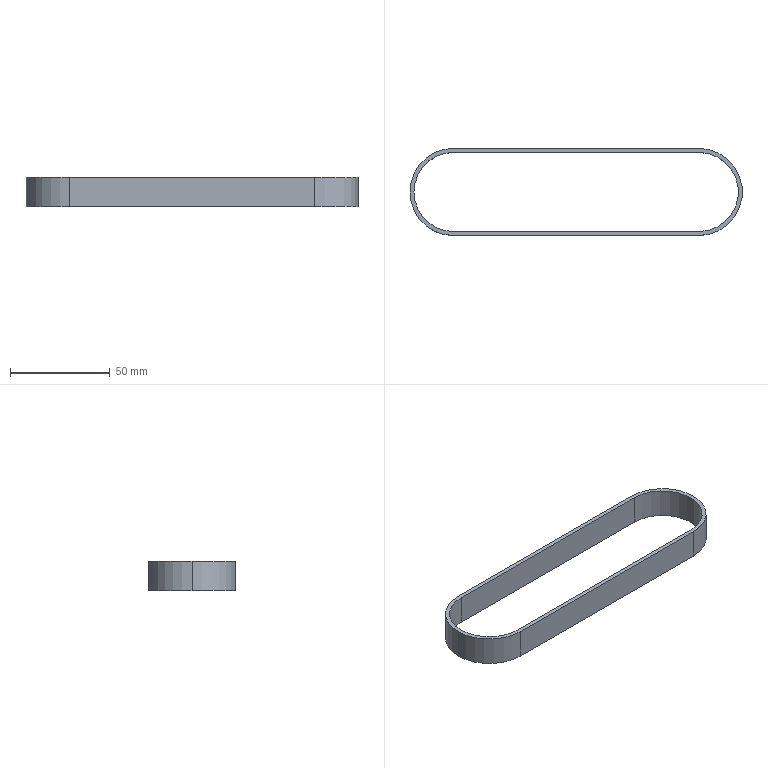Part | STEP file | C-HTBN370S5M-150 | 1 solid | 12 faces | box 166.79 x 43.79 x 15 mm | volume 11319 mm3 | cylinder 6 | plane 6 | commonest cylinder face diameters 39.79 x3 43.79 x3
STEP:
#1=CARTESIAN_POINT('',(0.,0.,0.));
#2=DIRECTION('',(0.,0.,1.));
#3=DIRECTION('',(1.,0.,0.));
#4=AXIS2_PLACEMENT_3D('',#1,#2,#3);
#5=CARTESIAN_POINT('',(-234.384,164.152,7.5));
#6=VERTEX_POINT('',#5);
#7=CARTESIAN_POINT('',(-234.384,164.152,-7.5));
#8=VERTEX_POINT('',#7);
#9=CARTESIAN_POINT('',(-234.384,164.152,7.5));
#10=DIRECTION('',(0.,0.,-1.));
#11=VECTOR('',#10,1.);
#12=LINE('',#9,#11);
#13=CARTESIAN_POINT('',(-234.384,144.257,7.5));
#14=DIRECTION('',(0.,0.,-1.));
#15=DIRECTION('',(-1.,0.,0.));
#16=AXIS2_PLACEMENT_3D('',#13,#14,#15);
#17=CYLINDRICAL_SURFACE('',#16,19.895);
#18=CARTESIAN_POINT('',(1.571,0.));
#19=DIRECTION('',(0.,1.));
#20=VECTOR('',#19,1.);
#21=LINE('',#18,#20);
#22=(GEOMETRIC_REPRESENTATION_CONTEXT(2)PARAMETRIC_REPRESENTATION_CONTEXT()REPRESENTATION_CONTEXT('',''));
#23=DEFINITIONAL_REPRESENTATION('',(#21),#22);
#24=PCURVE('',#17,#23);
#25=CARTESIAN_POINT('',(-234.384,164.152,7.5));
#26=DIRECTION('',(0.,-1.,0.));
#27=DIRECTION('',(0.,0.,-1.));
#28=AXIS2_PLACEMENT_3D('',#25,#26,#27);
#29=PLANE('',#28);
#30=CARTESIAN_POINT('',(0.,0.));
#31=DIRECTION('',(1.,0.));
#32=VECTOR('',#31,1.);
#33=LINE('',#30,#32);
#34=(GEOMETRIC_REPRESENTATION_CONTEXT(2)PARAMETRIC_REPRESENTATION_CONTEXT()REPRESENTATION_CONTEXT('',''));
#35=DEFINITIONAL_REPRESENTATION('',(#33),#34);
#36=PCURVE('',#29,#35);
#37=SURFACE_CURVE('',#12,(#24,#36),.PCURVE_S1.);
#38=EDGE_CURVE('',#6,#8,#37,.T.);
#39=ORIENTED_EDGE('',*,*,#38,.T.);
#40=CARTESIAN_POINT('',(-254.279,144.257,-7.5));
#41=VERTEX_POINT('',#40);
#42=CARTESIAN_POINT('',(-234.384,144.257,-7.5));
#43=DIRECTION('',(0.,0.,1.));
#44=DIRECTION('',(1.,0.,0.));
#45=AXIS2_PLACEMENT_3D('',#42,#43,#44);
#46=CIRCLE('',#45,19.895);
#47=CARTESIAN_POINT('',(3.142,15.));
#48=DIRECTION('',(-1.,0.));
#49=VECTOR('',#48,1.);
#50=LINE('',#47,#49);
#51=(GEOMETRIC_REPRESENTATION_CONTEXT(2)PARAMETRIC_REPRESENTATION_CONTEXT()REPRESENTATION_CONTEXT('',''));
#52=DEFINITIONAL_REPRESENTATION('',(#50),#51);
#53=PCURVE('',#17,#52);
#54=CARTESIAN_POINT('',(-234.384,144.257,-7.5));
#55=DIRECTION('',(0.,0.,1.));
#56=DIRECTION('',(1.,0.,0.));
#57=AXIS2_PLACEMENT_3D('',#54,#55,#56);
#58=PLANE('',#57);
#59=CARTESIAN_POINT('',(0.,0.));
#60=DIRECTION('',(1.,0.));
#61=AXIS2_PLACEMENT_2D('',#59,#60);
#62=CIRCLE('',#61,19.895);
#63=(GEOMETRIC_REPRESENTATION_CONTEXT(2)PARAMETRIC_REPRESENTATION_CONTEXT()REPRESENTATION_CONTEXT('',''));
#64=DEFINITIONAL_REPRESENTATION('',(#62),#63);
#65=PCURVE('',#58,#64);
#66=SURFACE_CURVE('',#46,(#53,#65),.PCURVE_S1.);
#67=EDGE_CURVE('',#8,#41,#66,.T.);
#68=ORIENTED_EDGE('',*,*,#67,.T.);
#69=CARTESIAN_POINT('',(-254.279,144.257,7.5));
#70=VERTEX_POINT('',#69);
#71=CARTESIAN_POINT('',(-254.279,144.257,7.5));
#72=DIRECTION('',(0.,0.,-1.));
#73=VECTOR('',#72,1.);
#74=LINE('',#71,#73);
#75=CARTESIAN_POINT('',(0.,0.));
#76=DIRECTION('',(0.,1.));
#77=VECTOR('',#76,1.);
#78=LINE('',#75,#77);
#79=(GEOMETRIC_REPRESENTATION_CONTEXT(2)PARAMETRIC_REPRESENTATION_CONTEXT()REPRESENTATION_CONTEXT('',''));
#80=DEFINITIONAL_REPRESENTATION('',(#78),#79);
#81=PCURVE('',#17,#80);
#82=CARTESIAN_POINT('',(-234.384,144.257,7.5));
#83=DIRECTION('',(0.,0.,-1.));
#84=DIRECTION('',(-1.,0.,0.));
#85=AXIS2_PLACEMENT_3D('',#82,#83,#84);
#86=CYLINDRICAL_SURFACE('',#85,19.895);
#87=CARTESIAN_POINT('',(6.283,0.));
#88=DIRECTION('',(0.,1.));
#89=VECTOR('',#88,1.);
#90=LINE('',#87,#89);
#91=(GEOMETRIC_REPRESENTATION_CONTEXT(2)PARAMETRIC_REPRESENTATION_CONTEXT()REPRESENTATION_CONTEXT('',''));
#92=DEFINITIONAL_REPRESENTATION('',(#90),#91);
#93=PCURVE('',#86,#92);
#94=SURFACE_CURVE('',#74,(#81,#93),.PCURVE_S1.);
#95=EDGE_CURVE('',#70,#41,#94,.T.);
#96=ORIENTED_EDGE('',*,*,#95,.F.);
#97=CARTESIAN_POINT('',(-234.384,144.257,7.5));
#98=DIRECTION('',(0.,0.,1.));
#99=DIRECTION('',(1.,0.,0.));
#100=AXIS2_PLACEMENT_3D('',#97,#98,#99);
#101=CIRCLE('',#100,19.895);
#102=CARTESIAN_POINT('',(3.142,0.));
#103=DIRECTION('',(-1.,0.));
#104=VECTOR('',#103,1.);
#105=LINE('',#102,#104);
#106=(GEOMETRIC_REPRESENTATION_CONTEXT(2)PARAMETRIC_REPRESENTATION_CONTEXT()REPRESENTATION_CONTEXT('',''));
#107=DEFINITIONAL_REPRESENTATION('',(#105),#106);
#108=PCURVE('',#17,#107);
#109=CARTESIAN_POINT('',(-234.384,144.257,7.5));
#110=DIRECTION('',(0.,0.,1.));
#111=DIRECTION('',(1.,0.,0.));
#112=AXIS2_PLACEMENT_3D('',#109,#110,#111);
#113=PLANE('',#112);
#114=CARTESIAN_POINT('',(0.,0.));
#115=DIRECTION('',(1.,0.));
#116=AXIS2_PLACEMENT_2D('',#114,#115);
#117=CIRCLE('',#116,19.895);
#118=(GEOMETRIC_REPRESENTATION_CONTEXT(2)PARAMETRIC_REPRESENTATION_CONTEXT()REPRESENTATION_CONTEXT('',''));
#119=DEFINITIONAL_REPRESENTATION('',(#117),#118);
#120=PCURVE('',#113,#119);
#121=SURFACE_CURVE('',#101,(#108,#120),.PCURVE_S1.);
#122=EDGE_CURVE('',#6,#70,#121,.T.);
#123=ORIENTED_EDGE('',*,*,#122,.F.);
#124=EDGE_LOOP('',(#39,#68,#96,#123));
#125=FACE_BOUND('',#124,.F.);
#126=ADVANCED_FACE('',(#125),#17,.F.);
#127=CARTESIAN_POINT('',(-256.279,144.257,7.5));
#128=VERTEX_POINT('',#127);
#129=CARTESIAN_POINT('',(-234.384,122.362,7.5));
#130=VERTEX_POINT('',#129);
#131=CARTESIAN_POINT('',(-234.384,144.257,7.5));
#132=DIRECTION('',(0.,0.,1.));
#133=DIRECTION('',(1.,0.,0.));
#134=AXIS2_PLACEMENT_3D('',#131,#132,#133);
#135=CIRCLE('',#134,21.895);
#136=CARTESIAN_POINT('',(-234.384,144.257,7.5));
#137=DIRECTION('',(0.,0.,-1.));
#138=DIRECTION('',(-1.,0.,0.));
#139=AXIS2_PLACEMENT_3D('',#136,#137,#138);
#140=CYLINDRICAL_SURFACE('',#139,21.895);
#141=CARTESIAN_POINT('',(9.425,0.));
#142=DIRECTION('',(-1.,0.));
#143=VECTOR('',#142,1.);
#144=LINE('',#141,#143);
#145=(GEOMETRIC_REPRESENTATION_CONTEXT(2)PARAMETRIC_REPRESENTATION_CONTEXT()REPRESENTATION_CONTEXT('',''));
#146=DEFINITIONAL_REPRESENTATION('',(#144),#145);
#147=PCURVE('',#140,#146);
#148=CARTESIAN_POINT('',(0.,0.));
#149=DIRECTION('',(1.,0.));
#150=AXIS2_PLACEMENT_2D('',#148,#149);
#151=CIRCLE('',#150,21.895);
#152=(GEOMETRIC_REPRESENTATION_CONTEXT(2)PARAMETRIC_REPRESENTATION_CONTEXT()REPRESENTATION_CONTEXT('',''));
#153=DEFINITIONAL_REPRESENTATION('',(#151),#152);
#154=PCURVE('',#113,#153);
#155=SURFACE_CURVE('',#135,(#147,#154),.PCURVE_S1.);
#156=EDGE_CURVE('',#128,#130,#155,.T.);
#157=ORIENTED_EDGE('',*,*,#156,.F.);
#158=CARTESIAN_POINT('',(-256.279,144.257,-7.5));
#159=VERTEX_POINT('',#158);
#160=CARTESIAN_POINT('',(-256.279,144.257,7.5));
#161=DIRECTION('',(0.,0.,-1.));
#162=VECTOR('',#161,1.);
#163=LINE('',#160,#162);
#164=CARTESIAN_POINT('',(6.283,0.));
#165=DIRECTION('',(0.,1.));
#166=VECTOR('',#165,1.);
#167=LINE('',#164,#166);
#168=(GEOMETRIC_REPRESENTATION_CONTEXT(2)PARAMETRIC_REPRESENTATION_CONTEXT()REPRESENTATION_CONTEXT('',''));
#169=DEFINITIONAL_REPRESENTATION('',(#167),#168);
#170=PCURVE('',#140,#169);
#171=CARTESIAN_POINT('',(-234.384,144.257,7.5));
#172=DIRECTION('',(0.,0.,-1.));
#173=DIRECTION('',(-1.,0.,0.));
#174=AXIS2_PLACEMENT_3D('',#171,#172,#173);
#175=CYLINDRICAL_SURFACE('',#174,21.895);
#176=CARTESIAN_POINT('',(0.,0.));
#177=DIRECTION('',(0.,1.));
#178=VECTOR('',#177,1.);
#179=LINE('',#176,#178);
#180=(GEOMETRIC_REPRESENTATION_CONTEXT(2)PARAMETRIC_REPRESENTATION_CONTEXT()REPRESENTATION_CONTEXT('',''));
#181=DEFINITIONAL_REPRESENTATION('',(#179),#180);
#182=PCURVE('',#175,#181);
#183=SURFACE_CURVE('',#163,(#170,#182),.PCURVE_S1.);
#184=EDGE_CURVE('',#128,#159,#183,.T.);
#185=ORIENTED_EDGE('',*,*,#184,.T.);
#186=CARTESIAN_POINT('',(-234.384,122.362,-7.5));
#187=VERTEX_POINT('',#186);
#188=CARTESIAN_POINT('',(-234.384,144.257,-7.5));
#189=DIRECTION('',(0.,0.,1.));
#190=DIRECTION('',(1.,0.,0.));
#191=AXIS2_PLACEMENT_3D('',#188,#189,#190);
#192=CIRCLE('',#191,21.895);
#193=CARTESIAN_POINT('',(9.425,15.));
#194=DIRECTION('',(-1.,0.));
#195=VECTOR('',#194,1.);
#196=LINE('',#193,#195);
#197=(GEOMETRIC_REPRESENTATION_CONTEXT(2)PARAMETRIC_REPRESENTATION_CONTEXT()REPRESENTATION_CONTEXT('',''));
#198=DEFINITIONAL_REPRESENTATION('',(#196),#197);
#199=PCURVE('',#140,#198);
#200=CARTESIAN_POINT('',(0.,0.));
#201=DIRECTION('',(1.,0.));
#202=AXIS2_PLACEMENT_2D('',#200,#201);
#203=CIRCLE('',#202,21.895);
#204=(GEOMETRIC_REPRESENTATION_CONTEXT(2)PARAMETRIC_REPRESENTATION_CONTEXT()REPRESENTATION_CONTEXT('',''));
#205=DEFINITIONAL_REPRESENTATION('',(#203),#204);
#206=PCURVE('',#58,#205);
#207=SURFACE_CURVE('',#192,(#199,#206),.PCURVE_S1.);
#208=EDGE_CURVE('',#159,#187,#207,.T.);
#209=ORIENTED_EDGE('',*,*,#208,.T.);
#210=CARTESIAN_POINT('',(-234.384,122.362,7.5));
#211=DIRECTION('',(0.,0.,-1.));
#212=VECTOR('',#211,1.);
#213=LINE('',#210,#212);
#214=CARTESIAN_POINT('',(4.712,0.));
#215=DIRECTION('',(0.,1.));
#216=VECTOR('',#215,1.);
#217=LINE('',#214,#216);
#218=(GEOMETRIC_REPRESENTATION_CONTEXT(2)PARAMETRIC_REPRESENTATION_CONTEXT()REPRESENTATION_CONTEXT('',''));
#219=DEFINITIONAL_REPRESENTATION('',(#217),#218);
#220=PCURVE('',#140,#219);
#221=CARTESIAN_POINT('',(-234.384,122.362,7.5));
#222=DIRECTION('',(0.,1.,0.));
#223=DIRECTION('',(-1.,0.,0.));
#224=AXIS2_PLACEMENT_3D('',#221,#222,#223);
#225=PLANE('',#224);
#226=CARTESIAN_POINT('',(0.,0.));
#227=DIRECTION('',(0.,-1.));
#228=VECTOR('',#227,1.);
#229=LINE('',#226,#228);
#230=(GEOMETRIC_REPRESENTATION_CONTEXT(2)PARAMETRIC_REPRESENTATION_CONTEXT()REPRESENTATION_CONTEXT('',''));
#231=DEFINITIONAL_REPRESENTATION('',(#229),#230);
#232=PCURVE('',#225,#231);
#233=SURFACE_CURVE('',#213,(#220,#232),.PCURVE_S1.);
#234=EDGE_CURVE('',#130,#187,#233,.T.);
#235=ORIENTED_EDGE('',*,*,#234,.F.);
#236=EDGE_LOOP('',(#157,#185,#209,#235));
#237=FACE_BOUND('',#236,.T.);
#238=ADVANCED_FACE('',(#237),#140,.T.);
#239=CARTESIAN_POINT('',(-234.384,166.152,7.5));
#240=VERTEX_POINT('',#239);
#241=CARTESIAN_POINT('',(-234.384,144.257,7.5));
#242=DIRECTION('',(0.,0.,1.));
#243=DIRECTION('',(1.,0.,0.));
#244=AXIS2_PLACEMENT_3D('',#241,#242,#243);
#245=CIRCLE('',#244,21.895);
#246=CARTESIAN_POINT('',(0.,0.));
#247=DIRECTION('',(1.,0.));
#248=AXIS2_PLACEMENT_2D('',#246,#247);
#249=CIRCLE('',#248,21.895);
#250=(GEOMETRIC_REPRESENTATION_CONTEXT(2)PARAMETRIC_REPRESENTATION_CONTEXT()REPRESENTATION_CONTEXT('',''));
#251=DEFINITIONAL_REPRESENTATION('',(#249),#250);
#252=PCURVE('',#113,#251);
#253=CARTESIAN_POINT('',(3.142,0.));
#254=DIRECTION('',(-1.,0.));
#255=VECTOR('',#254,1.);
#256=LINE('',#253,#255);
#257=(GEOMETRIC_REPRESENTATION_CONTEXT(2)PARAMETRIC_REPRESENTATION_CONTEXT()REPRESENTATION_CONTEXT('',''));
#258=DEFINITIONAL_REPRESENTATION('',(#256),#257);
#259=PCURVE('',#175,#258);
#260=SURFACE_CURVE('',#245,(#252,#259),.PCURVE_S1.);
#261=EDGE_CURVE('',#240,#128,#260,.T.);
#262=ORIENTED_EDGE('',*,*,#261,.T.);
#263=ORIENTED_EDGE('',*,*,#156,.T.);
#264=CARTESIAN_POINT('',(-111.384,122.362,7.5));
#265=VERTEX_POINT('',#264);
#266=CARTESIAN_POINT('',(-234.384,122.362,7.5));
#267=DIRECTION('',(1.,0.,0.));
#268=VECTOR('',#267,1.);
#269=LINE('',#266,#268);
#270=CARTESIAN_POINT('',(0.,-21.895));
#271=DIRECTION('',(1.,0.));
#272=VECTOR('',#271,1.);
#273=LINE('',#270,#272);
#274=(GEOMETRIC_REPRESENTATION_CONTEXT(2)PARAMETRIC_REPRESENTATION_CONTEXT()REPRESENTATION_CONTEXT('',''));
#275=DEFINITIONAL_REPRESENTATION('',(#273),#274);
#276=PCURVE('',#113,#275);
#277=CARTESIAN_POINT('',(0.,0.));
#278=DIRECTION('',(-1.,0.));
#279=VECTOR('',#278,1.);
#280=LINE('',#277,#279);
#281=(GEOMETRIC_REPRESENTATION_CONTEXT(2)PARAMETRIC_REPRESENTATION_CONTEXT()REPRESENTATION_CONTEXT('',''));
#282=DEFINITIONAL_REPRESENTATION('',(#280),#281);
#283=PCURVE('',#225,#282);
#284=SURFACE_CURVE('',#269,(#276,#283),.PCURVE_S1.);
#285=EDGE_CURVE('',#130,#265,#284,.T.);
#286=ORIENTED_EDGE('',*,*,#285,.T.);
#287=CARTESIAN_POINT('',(-111.384,166.152,7.5));
#288=VERTEX_POINT('',#287);
#289=CARTESIAN_POINT('',(-111.384,144.257,7.5));
#290=DIRECTION('',(0.,0.,1.));
#291=DIRECTION('',(1.,0.,0.));
#292=AXIS2_PLACEMENT_3D('',#289,#290,#291);
#293=CIRCLE('',#292,21.895);
#294=CARTESIAN_POINT('',(123.,0.));
#295=DIRECTION('',(1.,0.));
#296=AXIS2_PLACEMENT_2D('',#294,#295);
#297=CIRCLE('',#296,21.895);
#298=(GEOMETRIC_REPRESENTATION_CONTEXT(2)PARAMETRIC_REPRESENTATION_CONTEXT()REPRESENTATION_CONTEXT('',''));
#299=DEFINITIONAL_REPRESENTATION('',(#297),#298);
#300=PCURVE('',#113,#299);
#301=CARTESIAN_POINT('',(-111.384,144.257,7.5));
#302=DIRECTION('',(0.,0.,-1.));
#303=DIRECTION('',(-1.,0.,0.));
#304=AXIS2_PLACEMENT_3D('',#301,#302,#303);
#305=CYLINDRICAL_SURFACE('',#304,21.895);
#306=CARTESIAN_POINT('',(9.425,0.));
#307=DIRECTION('',(-1.,0.));
#308=VECTOR('',#307,1.);
#309=LINE('',#306,#308);
#310=(GEOMETRIC_REPRESENTATION_CONTEXT(2)PARAMETRIC_REPRESENTATION_CONTEXT()REPRESENTATION_CONTEXT('',''));
#311=DEFINITIONAL_REPRESENTATION('',(#309),#310);
#312=PCURVE('',#305,#311);
#313=SURFACE_CURVE('',#293,(#300,#312),.PCURVE_S1.);
#314=EDGE_CURVE('',#265,#288,#313,.T.);
#315=ORIENTED_EDGE('',*,*,#314,.T.);
#316=CARTESIAN_POINT('',(-234.384,166.152,7.5));
#317=DIRECTION('',(-1.,0.,0.));
#318=VECTOR('',#317,1.);
#319=LINE('',#316,#318);
#320=CARTESIAN_POINT('',(0.,21.895));
#321=DIRECTION('',(-1.,0.));
#322=VECTOR('',#321,1.);
#323=LINE('',#320,#322);
#324=(GEOMETRIC_REPRESENTATION_CONTEXT(2)PARAMETRIC_REPRESENTATION_CONTEXT()REPRESENTATION_CONTEXT('',''));
#325=DEFINITIONAL_REPRESENTATION('',(#323),#324);
#326=PCURVE('',#113,#325);
#327=CARTESIAN_POINT('',(-234.384,166.152,7.5));
#328=DIRECTION('',(0.,-1.,0.));
#329=DIRECTION('',(0.,0.,-1.));
#330=AXIS2_PLACEMENT_3D('',#327,#328,#329);
#331=PLANE('',#330);
#332=CARTESIAN_POINT('',(0.,0.));
#333=DIRECTION('',(0.,-1.));
#334=VECTOR('',#333,1.);
#335=LINE('',#332,#334);
#336=(GEOMETRIC_REPRESENTATION_CONTEXT(2)PARAMETRIC_REPRESENTATION_CONTEXT()REPRESENTATION_CONTEXT('',''));
#337=DEFINITIONAL_REPRESENTATION('',(#335),#336);
#338=PCURVE('',#331,#337);
#339=SURFACE_CURVE('',#319,(#326,#338),.PCURVE_S1.);
#340=EDGE_CURVE('',#288,#240,#339,.T.);
#341=ORIENTED_EDGE('',*,*,#340,.T.);
#342=EDGE_LOOP('',(#262,#263,#286,#315,#341));
#343=FACE_BOUND('',#342,.T.);
#344=CARTESIAN_POINT('',(-234.384,124.362,7.5));
#345=VERTEX_POINT('',#344);
#346=CARTESIAN_POINT('',(-111.384,124.362,7.5));
#347=VERTEX_POINT('',#346);
#348=CARTESIAN_POINT('',(-234.384,124.362,7.5));
#349=DIRECTION('',(1.,0.,0.));
#350=VECTOR('',#349,1.);
#351=LINE('',#348,#350);
#352=CARTESIAN_POINT('',(0.,-19.895));
#353=DIRECTION('',(1.,0.));
#354=VECTOR('',#353,1.);
#355=LINE('',#352,#354);
#356=(GEOMETRIC_REPRESENTATION_CONTEXT(2)PARAMETRIC_REPRESENTATION_CONTEXT()REPRESENTATION_CONTEXT('',''));
#357=DEFINITIONAL_REPRESENTATION('',(#355),#356);
#358=PCURVE('',#113,#357);
#359=CARTESIAN_POINT('',(-234.384,124.362,7.5));
#360=DIRECTION('',(0.,1.,0.));
#361=DIRECTION('',(-1.,0.,0.));
#362=AXIS2_PLACEMENT_3D('',#359,#360,#361);
#363=PLANE('',#362);
#364=CARTESIAN_POINT('',(0.,0.));
#365=DIRECTION('',(-1.,0.));
#366=VECTOR('',#365,1.);
#367=LINE('',#364,#366);
#368=(GEOMETRIC_REPRESENTATION_CONTEXT(2)PARAMETRIC_REPRESENTATION_CONTEXT()REPRESENTATION_CONTEXT('',''));
#369=DEFINITIONAL_REPRESENTATION('',(#367),#368);
#370=PCURVE('',#363,#369);
#371=SURFACE_CURVE('',#351,(#358,#370),.PCURVE_S1.);
#372=EDGE_CURVE('',#345,#347,#371,.T.);
#373=ORIENTED_EDGE('',*,*,#372,.F.);
#374=CARTESIAN_POINT('',(-234.384,144.257,7.5));
#375=DIRECTION('',(0.,0.,1.));
#376=DIRECTION('',(1.,0.,0.));
#377=AXIS2_PLACEMENT_3D('',#374,#375,#376);
#378=CIRCLE('',#377,19.895);
#379=CARTESIAN_POINT('',(0.,0.));
#380=DIRECTION('',(1.,0.));
#381=AXIS2_PLACEMENT_2D('',#379,#380);
#382=CIRCLE('',#381,19.895);
#383=(GEOMETRIC_REPRESENTATION_CONTEXT(2)PARAMETRIC_REPRESENTATION_CONTEXT()REPRESENTATION_CONTEXT('',''));
#384=DEFINITIONAL_REPRESENTATION('',(#382),#383);
#385=PCURVE('',#113,#384);
#386=CARTESIAN_POINT('',(9.425,0.));
#387=DIRECTION('',(-1.,0.));
#388=VECTOR('',#387,1.);
#389=LINE('',#386,#388);
#390=(GEOMETRIC_REPRESENTATION_CONTEXT(2)PARAMETRIC_REPRESENTATION_CONTEXT()REPRESENTATION_CONTEXT('',''));
#391=DEFINITIONAL_REPRESENTATION('',(#389),#390);
#392=PCURVE('',#86,#391);
#393=SURFACE_CURVE('',#378,(#385,#392),.PCURVE_S1.);
#394=EDGE_CURVE('',#70,#345,#393,.T.);
#395=ORIENTED_EDGE('',*,*,#394,.F.);
#396=ORIENTED_EDGE('',*,*,#122,.F.);
#397=CARTESIAN_POINT('',(-111.384,164.152,7.5));
#398=VERTEX_POINT('',#397);
#399=CARTESIAN_POINT('',(-234.384,164.152,7.5));
#400=DIRECTION('',(-1.,0.,0.));
#401=VECTOR('',#400,1.);
#402=LINE('',#399,#401);
#403=CARTESIAN_POINT('',(0.,19.895));
#404=DIRECTION('',(-1.,0.));
#405=VECTOR('',#404,1.);
#406=LINE('',#403,#405);
#407=(GEOMETRIC_REPRESENTATION_CONTEXT(2)PARAMETRIC_REPRESENTATION_CONTEXT()REPRESENTATION_CONTEXT('',''));
#408=DEFINITIONAL_REPRESENTATION('',(#406),#407);
#409=PCURVE('',#113,#408);
#410=CARTESIAN_POINT('',(0.,0.));
#411=DIRECTION('',(0.,-1.));
#412=VECTOR('',#411,1.);
#413=LINE('',#410,#412);
#414=(GEOMETRIC_REPRESENTATION_CONTEXT(2)PARAMETRIC_REPRESENTATION_CONTEXT()REPRESENTATION_CONTEXT('',''));
#415=DEFINITIONAL_REPRESENTATION('',(#413),#414);
#416=PCURVE('',#29,#415);
#417=SURFACE_CURVE('',#402,(#409,#416),.PCURVE_S1.);
#418=EDGE_CURVE('',#398,#6,#417,.T.);
#419=ORIENTED_EDGE('',*,*,#418,.F.);
#420=CARTESIAN_POINT('',(-111.384,144.257,7.5));
#421=DIRECTION('',(0.,0.,1.));
#422=DIRECTION('',(1.,0.,0.));
#423=AXIS2_PLACEMENT_3D('',#420,#421,#422);
#424=CIRCLE('',#423,19.895);
#425=CARTESIAN_POINT('',(123.,0.));
#426=DIRECTION('',(1.,0.));
#427=AXIS2_PLACEMENT_2D('',#425,#426);
#428=CIRCLE('',#427,19.895);
#429=(GEOMETRIC_REPRESENTATION_CONTEXT(2)PARAMETRIC_REPRESENTATION_CONTEXT()REPRESENTATION_CONTEXT('',''));
#430=DEFINITIONAL_REPRESENTATION('',(#428),#429);
#431=PCURVE('',#113,#430);
#432=CARTESIAN_POINT('',(-111.384,144.257,7.5));
#433=DIRECTION('',(0.,0.,-1.));
#434=DIRECTION('',(-1.,0.,0.));
#435=AXIS2_PLACEMENT_3D('',#432,#433,#434);
#436=CYLINDRICAL_SURFACE('',#435,19.895);
#437=CARTESIAN_POINT('',(9.425,0.));
#438=DIRECTION('',(-1.,0.));
#439=VECTOR('',#438,1.);
#440=LINE('',#437,#439);
#441=(GEOMETRIC_REPRESENTATION_CONTEXT(2)PARAMETRIC_REPRESENTATION_CONTEXT()REPRESENTATION_CONTEXT('',''));
#442=DEFINITIONAL_REPRESENTATION('',(#440),#441);
#443=PCURVE('',#436,#442);
#444=SURFACE_CURVE('',#424,(#431,#443),.PCURVE_S1.);
#445=EDGE_CURVE('',#347,#398,#444,.T.);
#446=ORIENTED_EDGE('',*,*,#445,.F.);
#447=EDGE_LOOP('',(#373,#395,#396,#419,#446));
#448=FACE_BOUND('',#447,.T.);
#449=ADVANCED_FACE('',(#343,#448),#113,.T.);
#450=CARTESIAN_POINT('',(-234.384,166.152,-7.5));
#451=VERTEX_POINT('',#450);
#452=CARTESIAN_POINT('',(-234.384,144.257,-7.5));
#453=DIRECTION('',(0.,0.,1.));
#454=DIRECTION('',(1.,0.,0.));
#455=AXIS2_PLACEMENT_3D('',#452,#453,#454);
#456=CIRCLE('',#455,21.895);
#457=CARTESIAN_POINT('',(0.,0.));
#458=DIRECTION('',(1.,0.));
#459=AXIS2_PLACEMENT_2D('',#457,#458);
#460=CIRCLE('',#459,21.895);
#461=(GEOMETRIC_REPRESENTATION_CONTEXT(2)PARAMETRIC_REPRESENTATION_CONTEXT()REPRESENTATION_CONTEXT('',''));
#462=DEFINITIONAL_REPRESENTATION('',(#460),#461);
#463=PCURVE('',#58,#462);
#464=CARTESIAN_POINT('',(3.142,15.));
#465=DIRECTION('',(-1.,0.));
#466=VECTOR('',#465,1.);
#467=LINE('',#464,#466);
#468=(GEOMETRIC_REPRESENTATION_CONTEXT(2)PARAMETRIC_REPRESENTATION_CONTEXT()REPRESENTATION_CONTEXT('',''));
#469=DEFINITIONAL_REPRESENTATION('',(#467),#468);
#470=PCURVE('',#175,#469);
#471=SURFACE_CURVE('',#456,(#463,#470),.PCURVE_S1.);
#472=EDGE_CURVE('',#451,#159,#471,.T.);
#473=ORIENTED_EDGE('',*,*,#472,.F.);
#474=CARTESIAN_POINT('',(-111.384,166.152,-7.5));
#475=VERTEX_POINT('',#474);
#476=CARTESIAN_POINT('',(-234.384,166.152,-7.5));
#477=DIRECTION('',(-1.,0.,0.));
#478=VECTOR('',#477,1.);
#479=LINE('',#476,#478);
#480=CARTESIAN_POINT('',(0.,21.895));
#481=DIRECTION('',(-1.,0.));
#482=VECTOR('',#481,1.);
#483=LINE('',#480,#482);
#484=(GEOMETRIC_REPRESENTATION_CONTEXT(2)PARAMETRIC_REPRESENTATION_CONTEXT()REPRESENTATION_CONTEXT('',''));
#485=DEFINITIONAL_REPRESENTATION('',(#483),#484);
#486=PCURVE('',#58,#485);
#487=CARTESIAN_POINT('',(15.,0.));
#488=DIRECTION('',(0.,-1.));
#489=VECTOR('',#488,1.);
#490=LINE('',#487,#489);
#491=(GEOMETRIC_REPRESENTATION_CONTEXT(2)PARAMETRIC_REPRESENTATION_CONTEXT()REPRESENTATION_CONTEXT('',''));
#492=DEFINITIONAL_REPRESENTATION('',(#490),#491);
#493=PCURVE('',#331,#492);
#494=SURFACE_CURVE('',#479,(#486,#493),.PCURVE_S1.);
#495=EDGE_CURVE('',#475,#451,#494,.T.);
#496=ORIENTED_EDGE('',*,*,#495,.F.);
#497=CARTESIAN_POINT('',(-111.384,122.362,-7.5));
#498=VERTEX_POINT('',#497);
#499=CARTESIAN_POINT('',(-111.384,144.257,-7.5));
#500=DIRECTION('',(0.,0.,1.));
#501=DIRECTION('',(1.,0.,0.));
#502=AXIS2_PLACEMENT_3D('',#499,#500,#501);
#503=CIRCLE('',#502,21.895);
#504=CARTESIAN_POINT('',(123.,0.));
#505=DIRECTION('',(1.,0.));
#506=AXIS2_PLACEMENT_2D('',#504,#505);
#507=CIRCLE('',#506,21.895);
#508=(GEOMETRIC_REPRESENTATION_CONTEXT(2)PARAMETRIC_REPRESENTATION_CONTEXT()REPRESENTATION_CONTEXT('',''));
#509=DEFINITIONAL_REPRESENTATION('',(#507),#508);
#510=PCURVE('',#58,#509);
#511=CARTESIAN_POINT('',(9.425,15.));
#512=DIRECTION('',(-1.,0.));
#513=VECTOR('',#512,1.);
#514=LINE('',#511,#513);
#515=(GEOMETRIC_REPRESENTATION_CONTEXT(2)PARAMETRIC_REPRESENTATION_CONTEXT()REPRESENTATION_CONTEXT('',''));
#516=DEFINITIONAL_REPRESENTATION('',(#514),#515);
#517=PCURVE('',#305,#516);
#518=SURFACE_CURVE('',#503,(#510,#517),.PCURVE_S1.);
#519=EDGE_CURVE('',#498,#475,#518,.T.);
#520=ORIENTED_EDGE('',*,*,#519,.F.);
#521=CARTESIAN_POINT('',(-234.384,122.362,-7.5));
#522=DIRECTION('',(1.,0.,0.));
#523=VECTOR('',#522,1.);
#524=LINE('',#521,#523);
#525=CARTESIAN_POINT('',(0.,-21.895));
#526=DIRECTION('',(1.,0.));
#527=VECTOR('',#526,1.);
#528=LINE('',#525,#527);
#529=(GEOMETRIC_REPRESENTATION_CONTEXT(2)PARAMETRIC_REPRESENTATION_CONTEXT()REPRESENTATION_CONTEXT('',''));
#530=DEFINITIONAL_REPRESENTATION('',(#528),#529);
#531=PCURVE('',#58,#530);
#532=CARTESIAN_POINT('',(0.,-15.));
#533=DIRECTION('',(-1.,0.));
#534=VECTOR('',#533,1.);
#535=LINE('',#532,#534);
#536=(GEOMETRIC_REPRESENTATION_CONTEXT(2)PARAMETRIC_REPRESENTATION_CONTEXT()REPRESENTATION_CONTEXT('',''));
#537=DEFINITIONAL_REPRESENTATION('',(#535),#536);
#538=PCURVE('',#225,#537);
#539=SURFACE_CURVE('',#524,(#531,#538),.PCURVE_S1.);
#540=EDGE_CURVE('',#187,#498,#539,.T.);
#541=ORIENTED_EDGE('',*,*,#540,.F.);
#542=ORIENTED_EDGE('',*,*,#208,.F.);
#543=EDGE_LOOP('',(#473,#496,#520,#541,#542));
#544=FACE_BOUND('',#543,.T.);
#545=ORIENTED_EDGE('',*,*,#67,.T.);
#546=CARTESIAN_POINT('',(-234.384,124.362,-7.5));
#547=VERTEX_POINT('',#546);
#548=CARTESIAN_POINT('',(-234.384,144.257,-7.5));
#549=DIRECTION('',(0.,0.,1.));
#550=DIRECTION('',(1.,0.,0.));
#551=AXIS2_PLACEMENT_3D('',#548,#549,#550);
#552=CIRCLE('',#551,19.895);
#553=CARTESIAN_POINT('',(0.,0.));
#554=DIRECTION('',(1.,0.));
#555=AXIS2_PLACEMENT_2D('',#553,#554);
#556=CIRCLE('',#555,19.895);
#557=(GEOMETRIC_REPRESENTATION_CONTEXT(2)PARAMETRIC_REPRESENTATION_CONTEXT()REPRESENTATION_CONTEXT('',''));
#558=DEFINITIONAL_REPRESENTATION('',(#556),#557);
#559=PCURVE('',#58,#558);
#560=CARTESIAN_POINT('',(9.425,15.));
#561=DIRECTION('',(-1.,0.));
#562=VECTOR('',#561,1.);
#563=LINE('',#560,#562);
#564=(GEOMETRIC_REPRESENTATION_CONTEXT(2)PARAMETRIC_REPRESENTATION_CONTEXT()REPRESENTATION_CONTEXT('',''));
#565=DEFINITIONAL_REPRESENTATION('',(#563),#564);
#566=PCURVE('',#86,#565);
#567=SURFACE_CURVE('',#552,(#559,#566),.PCURVE_S1.);
#568=EDGE_CURVE('',#41,#547,#567,.T.);
#569=ORIENTED_EDGE('',*,*,#568,.T.);
#570=CARTESIAN_POINT('',(-111.384,124.362,-7.5));
#571=VERTEX_POINT('',#570);
#572=CARTESIAN_POINT('',(-234.384,124.362,-7.5));
#573=DIRECTION('',(1.,0.,0.));
#574=VECTOR('',#573,1.);
#575=LINE('',#572,#574);
#576=CARTESIAN_POINT('',(0.,-19.895));
#577=DIRECTION('',(1.,0.));
#578=VECTOR('',#577,1.);
#579=LINE('',#576,#578);
#580=(GEOMETRIC_REPRESENTATION_CONTEXT(2)PARAMETRIC_REPRESENTATION_CONTEXT()REPRESENTATION_CONTEXT('',''));
#581=DEFINITIONAL_REPRESENTATION('',(#579),#580);
#582=PCURVE('',#58,#581);
#583=CARTESIAN_POINT('',(0.,-15.));
#584=DIRECTION('',(-1.,0.));
#585=VECTOR('',#584,1.);
#586=LINE('',#583,#585);
#587=(GEOMETRIC_REPRESENTATION_CONTEXT(2)PARAMETRIC_REPRESENTATION_CONTEXT()REPRESENTATION_CONTEXT('',''));
#588=DEFINITIONAL_REPRESENTATION('',(#586),#587);
#589=PCURVE('',#363,#588);
#590=SURFACE_CURVE('',#575,(#582,#589),.PCURVE_S1.);
#591=EDGE_CURVE('',#547,#571,#590,.T.);
#592=ORIENTED_EDGE('',*,*,#591,.T.);
#593=CARTESIAN_POINT('',(-111.384,164.152,-7.5));
#594=VERTEX_POINT('',#593);
#595=CARTESIAN_POINT('',(-111.384,144.257,-7.5));
#596=DIRECTION('',(0.,0.,1.));
#597=DIRECTION('',(1.,0.,0.));
#598=AXIS2_PLACEMENT_3D('',#595,#596,#597);
#599=CIRCLE('',#598,19.895);
#600=CARTESIAN_POINT('',(123.,0.));
#601=DIRECTION('',(1.,0.));
#602=AXIS2_PLACEMENT_2D('',#600,#601);
#603=CIRCLE('',#602,19.895);
#604=(GEOMETRIC_REPRESENTATION_CONTEXT(2)PARAMETRIC_REPRESENTATION_CONTEXT()REPRESENTATION_CONTEXT('',''));
#605=DEFINITIONAL_REPRESENTATION('',(#603),#604);
#606=PCURVE('',#58,#605);
#607=CARTESIAN_POINT('',(9.425,15.));
#608=DIRECTION('',(-1.,0.));
#609=VECTOR('',#608,1.);
#610=LINE('',#607,#609);
#611=(GEOMETRIC_REPRESENTATION_CONTEXT(2)PARAMETRIC_REPRESENTATION_CONTEXT()REPRESENTATION_CONTEXT('',''));
#612=DEFINITIONAL_REPRESENTATION('',(#610),#611);
#613=PCURVE('',#436,#612);
#614=SURFACE_CURVE('',#599,(#606,#613),.PCURVE_S1.);
#615=EDGE_CURVE('',#571,#594,#614,.T.);
#616=ORIENTED_EDGE('',*,*,#615,.T.);
#617=CARTESIAN_POINT('',(-234.384,164.152,-7.5));
#618=DIRECTION('',(-1.,0.,0.));
#619=VECTOR('',#618,1.);
#620=LINE('',#617,#619);
#621=CARTESIAN_POINT('',(0.,19.895));
#622=DIRECTION('',(-1.,0.));
#623=VECTOR('',#622,1.);
#624=LINE('',#621,#623);
#625=(GEOMETRIC_REPRESENTATION_CONTEXT(2)PARAMETRIC_REPRESENTATION_CONTEXT()REPRESENTATION_CONTEXT('',''));
#626=DEFINITIONAL_REPRESENTATION('',(#624),#625);
#627=PCURVE('',#58,#626);
#628=CARTESIAN_POINT('',(15.,0.));
#629=DIRECTION('',(0.,-1.));
#630=VECTOR('',#629,1.);
#631=LINE('',#628,#630);
#632=(GEOMETRIC_REPRESENTATION_CONTEXT(2)PARAMETRIC_REPRESENTATION_CONTEXT()REPRESENTATION_CONTEXT('',''));
#633=DEFINITIONAL_REPRESENTATION('',(#631),#632);
#634=PCURVE('',#29,#633);
#635=SURFACE_CURVE('',#620,(#627,#634),.PCURVE_S1.);
#636=EDGE_CURVE('',#594,#8,#635,.T.);
#637=ORIENTED_EDGE('',*,*,#636,.T.);
#638=EDGE_LOOP('',(#545,#569,#592,#616,#637));
#639=FACE_BOUND('',#638,.T.);
#640=ADVANCED_FACE('',(#544,#639),#58,.F.);
#641=ORIENTED_EDGE('',*,*,#184,.F.);
#642=ORIENTED_EDGE('',*,*,#261,.F.);
#643=CARTESIAN_POINT('',(-234.384,166.152,7.5));
#644=DIRECTION('',(0.,0.,-1.));
#645=VECTOR('',#644,1.);
#646=LINE('',#643,#645);
#647=CARTESIAN_POINT('',(1.571,0.));
#648=DIRECTION('',(0.,1.));
#649=VECTOR('',#648,1.);
#650=LINE('',#647,#649);
#651=(GEOMETRIC_REPRESENTATION_CONTEXT(2)PARAMETRIC_REPRESENTATION_CONTEXT()REPRESENTATION_CONTEXT('',''));
#652=DEFINITIONAL_REPRESENTATION('',(#650),#651);
#653=PCURVE('',#175,#652);
#654=CARTESIAN_POINT('',(0.,0.));
#655=DIRECTION('',(1.,0.));
#656=VECTOR('',#655,1.);
#657=LINE('',#654,#656);
#658=(GEOMETRIC_REPRESENTATION_CONTEXT(2)PARAMETRIC_REPRESENTATION_CONTEXT()REPRESENTATION_CONTEXT('',''));
#659=DEFINITIONAL_REPRESENTATION('',(#657),#658);
#660=PCURVE('',#331,#659);
#661=SURFACE_CURVE('',#646,(#653,#660),.PCURVE_S1.);
#662=EDGE_CURVE('',#240,#451,#661,.T.);
#663=ORIENTED_EDGE('',*,*,#662,.T.);
#664=ORIENTED_EDGE('',*,*,#472,.T.);
#665=EDGE_LOOP('',(#641,#642,#663,#664));
#666=FACE_BOUND('',#665,.T.);
#667=ADVANCED_FACE('',(#666),#175,.T.);
#668=ORIENTED_EDGE('',*,*,#540,.T.);
#669=CARTESIAN_POINT('',(-111.384,122.362,7.5));
#670=DIRECTION('',(0.,0.,-1.));
#671=VECTOR('',#670,1.);
#672=LINE('',#669,#671);
#673=CARTESIAN_POINT('',(-123.,0.));
#674=DIRECTION('',(0.,-1.));
#675=VECTOR('',#674,1.);
#676=LINE('',#673,#675);
#677=(GEOMETRIC_REPRESENTATION_CONTEXT(2)PARAMETRIC_REPRESENTATION_CONTEXT()REPRESENTATION_CONTEXT('',''));
#678=DEFINITIONAL_REPRESENTATION('',(#676),#677);
#679=PCURVE('',#225,#678);
#680=CARTESIAN_POINT('',(4.712,0.));
#681=DIRECTION('',(0.,1.));
#682=VECTOR('',#681,1.);
#683=LINE('',#680,#682);
#684=(GEOMETRIC_REPRESENTATION_CONTEXT(2)PARAMETRIC_REPRESENTATION_CONTEXT()REPRESENTATION_CONTEXT('',''));
#685=DEFINITIONAL_REPRESENTATION('',(#683),#684);
#686=PCURVE('',#305,#685);
#687=SURFACE_CURVE('',#672,(#679,#686),.PCURVE_S1.);
#688=EDGE_CURVE('',#265,#498,#687,.T.);
#689=ORIENTED_EDGE('',*,*,#688,.F.);
#690=ORIENTED_EDGE('',*,*,#285,.F.);
#691=ORIENTED_EDGE('',*,*,#234,.T.);
#692=EDGE_LOOP('',(#668,#689,#690,#691));
#693=FACE_BOUND('',#692,.T.);
#694=ADVANCED_FACE('',(#693),#225,.F.);
#695=ORIENTED_EDGE('',*,*,#519,.T.);
#696=CARTESIAN_POINT('',(-111.384,166.152,7.5));
#697=DIRECTION('',(0.,0.,-1.));
#698=VECTOR('',#697,1.);
#699=LINE('',#696,#698);
#700=CARTESIAN_POINT('',(1.571,0.));
#701=DIRECTION('',(0.,1.));
#702=VECTOR('',#701,1.);
#703=LINE('',#700,#702);
#704=(GEOMETRIC_REPRESENTATION_CONTEXT(2)PARAMETRIC_REPRESENTATION_CONTEXT()REPRESENTATION_CONTEXT('',''));
#705=DEFINITIONAL_REPRESENTATION('',(#703),#704);
#706=PCURVE('',#305,#705);
#707=CARTESIAN_POINT('',(0.,123.));
#708=DIRECTION('',(1.,0.));
#709=VECTOR('',#708,1.);
#710=LINE('',#707,#709);
#711=(GEOMETRIC_REPRESENTATION_CONTEXT(2)PARAMETRIC_REPRESENTATION_CONTEXT()REPRESENTATION_CONTEXT('',''));
#712=DEFINITIONAL_REPRESENTATION('',(#710),#711);
#713=PCURVE('',#331,#712);
#714=SURFACE_CURVE('',#699,(#706,#713),.PCURVE_S1.);
#715=EDGE_CURVE('',#288,#475,#714,.T.);
#716=ORIENTED_EDGE('',*,*,#715,.F.);
#717=ORIENTED_EDGE('',*,*,#314,.F.);
#718=ORIENTED_EDGE('',*,*,#688,.T.);
#719=EDGE_LOOP('',(#695,#716,#717,#718));
#720=FACE_BOUND('',#719,.T.);
#721=ADVANCED_FACE('',(#720),#305,.T.);
#722=ORIENTED_EDGE('',*,*,#495,.T.);
#723=ORIENTED_EDGE('',*,*,#662,.F.);
#724=ORIENTED_EDGE('',*,*,#340,.F.);
#725=ORIENTED_EDGE('',*,*,#715,.T.);
#726=EDGE_LOOP('',(#722,#723,#724,#725));
#727=FACE_BOUND('',#726,.T.);
#728=ADVANCED_FACE('',(#727),#331,.F.);
#729=ORIENTED_EDGE('',*,*,#568,.T.);
#730=CARTESIAN_POINT('',(-234.384,124.362,7.5));
#731=DIRECTION('',(0.,0.,-1.));
#732=VECTOR('',#731,1.);
#733=LINE('',#730,#732);
#734=CARTESIAN_POINT('',(4.712,0.));
#735=DIRECTION('',(0.,1.));
#736=VECTOR('',#735,1.);
#737=LINE('',#734,#736);
#738=(GEOMETRIC_REPRESENTATION_CONTEXT(2)PARAMETRIC_REPRESENTATION_CONTEXT()REPRESENTATION_CONTEXT('',''));
#739=DEFINITIONAL_REPRESENTATION('',(#737),#738);
#740=PCURVE('',#86,#739);
#741=CARTESIAN_POINT('',(0.,0.));
#742=DIRECTION('',(0.,-1.));
#743=VECTOR('',#742,1.);
#744=LINE('',#741,#743);
#745=(GEOMETRIC_REPRESENTATION_CONTEXT(2)PARAMETRIC_REPRESENTATION_CONTEXT()REPRESENTATION_CONTEXT('',''));
#746=DEFINITIONAL_REPRESENTATION('',(#744),#745);
#747=PCURVE('',#363,#746);
#748=SURFACE_CURVE('',#733,(#740,#747),.PCURVE_S1.);
#749=EDGE_CURVE('',#345,#547,#748,.T.);
#750=ORIENTED_EDGE('',*,*,#749,.F.);
#751=ORIENTED_EDGE('',*,*,#394,.F.);
#752=ORIENTED_EDGE('',*,*,#95,.T.);
#753=EDGE_LOOP('',(#729,#750,#751,#752));
#754=FACE_BOUND('',#753,.F.);
#755=ADVANCED_FACE('',(#754),#86,.F.);
#756=ORIENTED_EDGE('',*,*,#591,.F.);
#757=ORIENTED_EDGE('',*,*,#749,.F.);
#758=ORIENTED_EDGE('',*,*,#372,.T.);
#759=CARTESIAN_POINT('',(-111.384,124.362,7.5));
#760=DIRECTION('',(0.,0.,-1.));
#761=VECTOR('',#760,1.);
#762=LINE('',#759,#761);
#763=CARTESIAN_POINT('',(-123.,0.));
#764=DIRECTION('',(0.,-1.));
#765=VECTOR('',#764,1.);
#766=LINE('',#763,#765);
#767=(GEOMETRIC_REPRESENTATION_CONTEXT(2)PARAMETRIC_REPRESENTATION_CONTEXT()REPRESENTATION_CONTEXT('',''));
#768=DEFINITIONAL_REPRESENTATION('',(#766),#767);
#769=PCURVE('',#363,#768);
#770=CARTESIAN_POINT('',(4.712,0.));
#771=DIRECTION('',(0.,1.));
#772=VECTOR('',#771,1.);
#773=LINE('',#770,#772);
#774=(GEOMETRIC_REPRESENTATION_CONTEXT(2)PARAMETRIC_REPRESENTATION_CONTEXT()REPRESENTATION_CONTEXT('',''));
#775=DEFINITIONAL_REPRESENTATION('',(#773),#774);
#776=PCURVE('',#436,#775);
#777=SURFACE_CURVE('',#762,(#769,#776),.PCURVE_S1.);
#778=EDGE_CURVE('',#347,#571,#777,.T.);
#779=ORIENTED_EDGE('',*,*,#778,.T.);
#780=EDGE_LOOP('',(#756,#757,#758,#779));
#781=FACE_BOUND('',#780,.T.);
#782=ADVANCED_FACE('',(#781),#363,.T.);
#783=CARTESIAN_POINT('',(-111.384,164.152,7.5));
#784=DIRECTION('',(0.,0.,-1.));
#785=VECTOR('',#784,1.);
#786=LINE('',#783,#785);
#787=CARTESIAN_POINT('',(1.571,0.));
#788=DIRECTION('',(0.,1.));
#789=VECTOR('',#788,1.);
#790=LINE('',#787,#789);
#791=(GEOMETRIC_REPRESENTATION_CONTEXT(2)PARAMETRIC_REPRESENTATION_CONTEXT()REPRESENTATION_CONTEXT('',''));
#792=DEFINITIONAL_REPRESENTATION('',(#790),#791);
#793=PCURVE('',#436,#792);
#794=CARTESIAN_POINT('',(0.,123.));
#795=DIRECTION('',(1.,0.));
#796=VECTOR('',#795,1.);
#797=LINE('',#794,#796);
#798=(GEOMETRIC_REPRESENTATION_CONTEXT(2)PARAMETRIC_REPRESENTATION_CONTEXT()REPRESENTATION_CONTEXT('',''));
#799=DEFINITIONAL_REPRESENTATION('',(#797),#798);
#800=PCURVE('',#29,#799);
#801=SURFACE_CURVE('',#786,(#793,#800),.PCURVE_S1.);
#802=EDGE_CURVE('',#398,#594,#801,.T.);
#803=ORIENTED_EDGE('',*,*,#802,.F.);
#804=ORIENTED_EDGE('',*,*,#445,.F.);
#805=ORIENTED_EDGE('',*,*,#778,.T.);
#806=ORIENTED_EDGE('',*,*,#615,.T.);
#807=EDGE_LOOP('',(#803,#804,#805,#806));
#808=FACE_BOUND('',#807,.F.);
#809=ADVANCED_FACE('',(#808),#436,.F.);
#810=ORIENTED_EDGE('',*,*,#636,.F.);
#811=ORIENTED_EDGE('',*,*,#802,.F.);
#812=ORIENTED_EDGE('',*,*,#418,.T.);
#813=ORIENTED_EDGE('',*,*,#38,.T.);
#814=EDGE_LOOP('',(#810,#811,#812,#813));
#815=FACE_BOUND('',#814,.T.);
#816=ADVANCED_FACE('',(#815),#29,.T.);
#817=CLOSED_SHELL('',(#126,#238,#449,#640,#667,#694,#721,#728,#755,#782,#809,#816));
#818=MANIFOLD_SOLID_BREP('',#817);
#819=(LENGTH_UNIT()NAMED_UNIT(*)SI_UNIT(.MILLI.,.METRE.));
#820=UNCERTAINTY_MEASURE_WITH_UNIT(LENGTH_MEASURE(0.0000001),#819,'','');
#821=(NAMED_UNIT(*)PLANE_ANGLE_UNIT()SI_UNIT($,.RADIAN.));
#822=(NAMED_UNIT(*)SI_UNIT($,.STERADIAN.)SOLID_ANGLE_UNIT());
#823=(GEOMETRIC_REPRESENTATION_CONTEXT(3)GLOBAL_UNCERTAINTY_ASSIGNED_CONTEXT((#820))GLOBAL_UNIT_ASSIGNED_CONTEXT((#819,#821,#822))REPRESENTATION_CONTEXT('',''));
#824=ADVANCED_BREP_SHAPE_REPRESENTATION('',(#4,#818),#823);